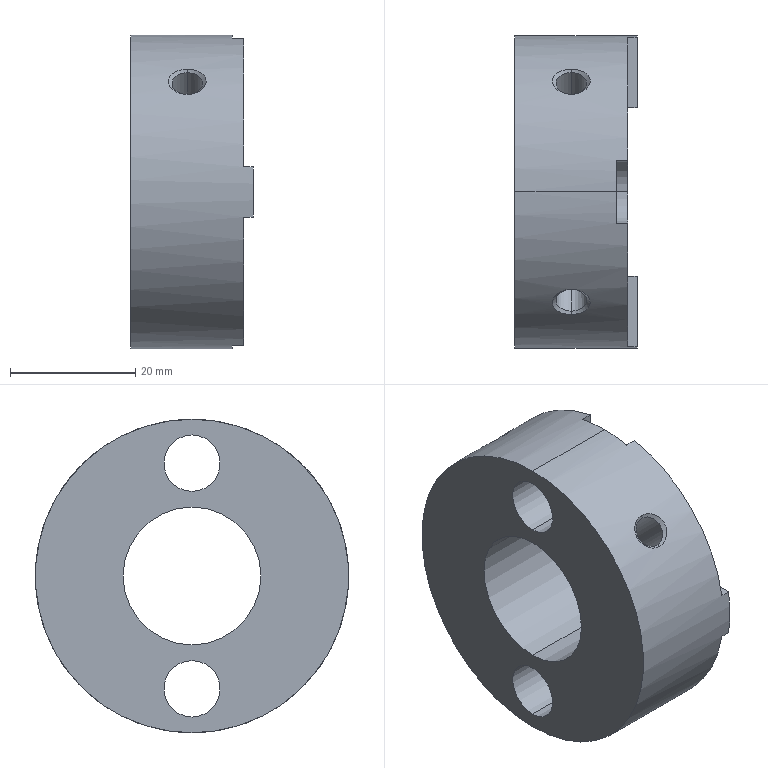Part | STEP file | _DBA01-D50-d20-e22-002 | 1 solid | 47 faces | box 19.5 x 50 x 50 mm | volume 25627 mm3 | cylinder 21 | plane 14 | cone 12 | commonest cylinder face diameters 4.134 x4 4.917 x4 9 x4 10.117 x3 22 x2 28 x2